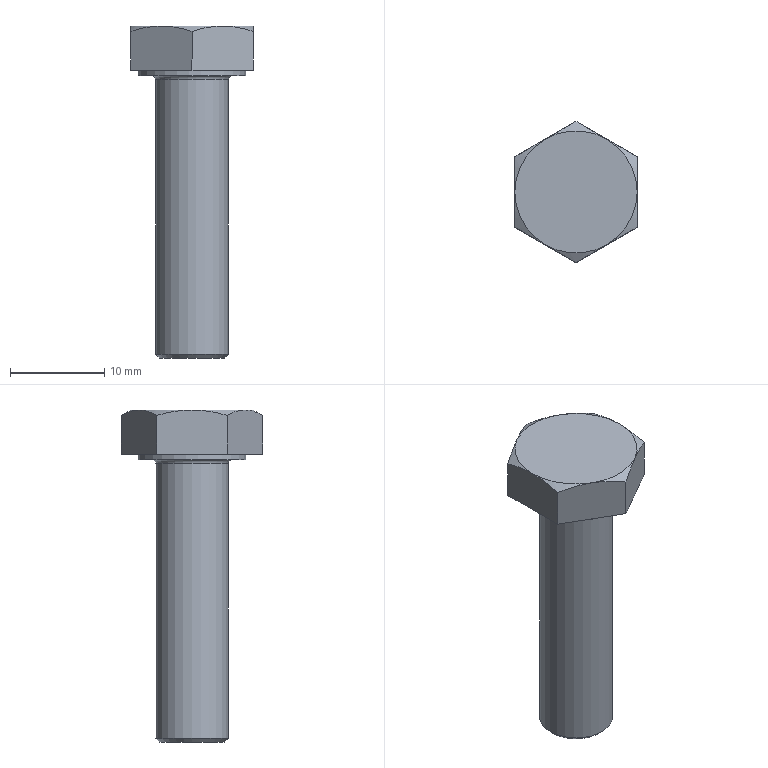Part | NX | features SKETCH 4, EXTRUDE 3, META 3, DATUM_CSYS 2, BLEND 1, CHAMFER 1, LINE 1, SWP104 1, SYMBOLIC_THREAD 1, THREADS 1 | 1 solid | 20 faces | box 13 x 15.011 x 35.3 mm | volume 2165 mm3 | plane 10 | cone 7 | cylinder 2 | torus 1 | commonest cylinder face diameters 7.76 x1 11.47 x1
STEP:
#1=CARTESIAN_POINT('',(4.28,0.,0.));
#2=VERTEX_POINT('',#1);
#3=CARTESIAN_POINT('',(0.,0.,0.));
#4=DIRECTION('',(0.,0.,1.));
#5=DIRECTION('',(1.,0.,0.));
#6=AXIS2_PLACEMENT_3D('',#3,#4,#5);
#7=CIRCLE('',#6,4.28);
#8=EDGE_CURVE('',#2,#2,#7,.T.);
#9=ORIENTED_EDGE('',*,*,#8,.T.);
#10=EDGE_LOOP('',(#9));
#11=FACE_BOUND('',#10,.T.);
#12=CARTESIAN_POINT('',(5.735,0.,0.));
#13=VERTEX_POINT('',#12);
#14=CARTESIAN_POINT('',(0.,0.,0.));
#15=DIRECTION('',(0.,0.,1.));
#16=DIRECTION('',(1.,0.,0.));
#17=AXIS2_PLACEMENT_3D('',#14,#15,#16);
#18=CIRCLE('',#17,5.735);
#19=EDGE_CURVE('',#13,#13,#18,.T.);
#20=ORIENTED_EDGE('',*,*,#19,.F.);
#21=EDGE_LOOP('',(#20));
#22=FACE_BOUND('',#21,.T.);
#23=CARTESIAN_POINT('',(0.,0.,0.));
#24=DIRECTION('',(0.,0.,1.));
#25=DIRECTION('',(1.,0.,0.));
#26=AXIS2_PLACEMENT_3D('',#23,#24,#25);
#27=PLANE('',#26);
#28=ADVANCED_FACE('',(#11,#22),#27,.F.);
#29=CARTESIAN_POINT('',(6.5,3.753,4.719));
#30=VERTEX_POINT('',#29);
#31=CARTESIAN_POINT('',(3.25,5.629,5.3));
#32=VERTEX_POINT('',#31);
#33=CARTESIAN_POINT('',(6.5,3.753,4.719));
#34=CARTESIAN_POINT('',(5.437,4.367,5.074));
#35=CARTESIAN_POINT('',(4.357,4.99,5.3));
#36=CARTESIAN_POINT('',(3.25,5.629,5.3));
#37=B_SPLINE_CURVE_WITH_KNOTS('',3,(#33,#34,#35,#36),.UNSPECIFIED.,.F.,.F.,(4,4),(0.000000238,0.003797),.UNSPECIFIED.);
#38=EDGE_CURVE('',#30,#32,#37,.T.);
#39=ORIENTED_EDGE('',*,*,#38,.F.);
#40=CARTESIAN_POINT('',(6.5,3.753,0.6));
#41=VERTEX_POINT('',#40);
#42=CARTESIAN_POINT('',(6.5,3.753,5.3));
#43=DIRECTION('',(0.,0.,-1.));
#44=VECTOR('',#43,1000.);
#45=LINE('',#42,#44);
#46=EDGE_CURVE('',#30,#41,#45,.T.);
#47=ORIENTED_EDGE('',*,*,#46,.T.);
#48=CARTESIAN_POINT('',(0.,7.506,0.6));
#49=VERTEX_POINT('',#48);
#50=CARTESIAN_POINT('',(0.,7.506,0.6));
#51=DIRECTION('',(0.866,-0.5,0.));
#52=VECTOR('',#51,1000.);
#53=LINE('',#50,#52);
#54=EDGE_CURVE('',#49,#41,#53,.T.);
#55=ORIENTED_EDGE('',*,*,#54,.F.);
#56=CARTESIAN_POINT('',(0.,7.506,4.719));
#57=VERTEX_POINT('',#56);
#58=CARTESIAN_POINT('',(0.,7.506,5.3));
#59=DIRECTION('',(0.,0.,-1.));
#60=VECTOR('',#59,1000.);
#61=LINE('',#58,#60);
#62=EDGE_CURVE('',#57,#49,#61,.T.);
#63=ORIENTED_EDGE('',*,*,#62,.F.);
#64=CARTESIAN_POINT('',(3.25,5.629,5.3));
#65=CARTESIAN_POINT('',(2.147,6.266,5.3));
#66=CARTESIAN_POINT('',(1.061,6.893,5.073));
#67=CARTESIAN_POINT('',(0.,7.506,4.719));
#68=B_SPLINE_CURVE_WITH_KNOTS('',3,(#64,#65,#66,#67),.UNSPECIFIED.,.F.,.F.,(4,4),(0.003797,0.00758),.UNSPECIFIED.);
#69=EDGE_CURVE('',#32,#57,#68,.T.);
#70=ORIENTED_EDGE('',*,*,#69,.F.);
#71=EDGE_LOOP('',(#39,#47,#55,#63,#70));
#72=FACE_BOUND('',#71,.T.);
#73=CARTESIAN_POINT('',(0.,7.506,5.3));
#74=DIRECTION('',(0.5,0.866,0.));
#75=DIRECTION('',(-0.866,0.5,0.));
#76=AXIS2_PLACEMENT_3D('',#73,#74,#75);
#77=PLANE('',#76);
#78=ADVANCED_FACE('',(#72),#77,.T.);
#79=CARTESIAN_POINT('',(6.5,-3.753,4.719));
#80=VERTEX_POINT('',#79);
#81=CARTESIAN_POINT('',(6.5,0.,5.3));
#82=VERTEX_POINT('',#81);
#83=CARTESIAN_POINT('',(6.5,-3.753,4.719));
#84=CARTESIAN_POINT('',(6.5,-2.532,5.072));
#85=CARTESIAN_POINT('',(6.5,-1.268,5.3));
#86=CARTESIAN_POINT('',(6.5,0.,5.3));
#87=B_SPLINE_CURVE_WITH_KNOTS('',3,(#83,#84,#85,#86),.UNSPECIFIED.,.F.,.F.,(4,4),(0.006695,0.01049),.UNSPECIFIED.);
#88=EDGE_CURVE('',#80,#82,#87,.T.);
#89=ORIENTED_EDGE('',*,*,#88,.F.);
#90=CARTESIAN_POINT('',(6.5,-3.753,0.6));
#91=VERTEX_POINT('',#90);
#92=CARTESIAN_POINT('',(6.5,-3.753,5.3));
#93=DIRECTION('',(0.,0.,-1.));
#94=VECTOR('',#93,1000.);
#95=LINE('',#92,#94);
#96=EDGE_CURVE('',#80,#91,#95,.T.);
#97=ORIENTED_EDGE('',*,*,#96,.T.);
#98=CARTESIAN_POINT('',(6.5,3.753,0.6));
#99=DIRECTION('',(0.,-1.,0.));
#100=VECTOR('',#99,1000.);
#101=LINE('',#98,#100);
#102=EDGE_CURVE('',#41,#91,#101,.T.);
#103=ORIENTED_EDGE('',*,*,#102,.F.);
#104=ORIENTED_EDGE('',*,*,#46,.F.);
#105=CARTESIAN_POINT('',(6.5,0.,5.3));
#106=CARTESIAN_POINT('',(6.5,1.269,5.3));
#107=CARTESIAN_POINT('',(6.5,2.539,5.07));
#108=CARTESIAN_POINT('',(6.5,3.753,4.719));
#109=B_SPLINE_CURVE_WITH_KNOTS('',3,(#105,#106,#107,#108),.UNSPECIFIED.,.F.,.F.,(4,4),(0.01049,0.01429),.UNSPECIFIED.);
#110=EDGE_CURVE('',#82,#30,#109,.T.);
#111=ORIENTED_EDGE('',*,*,#110,.F.);
#112=EDGE_LOOP('',(#89,#97,#103,#104,#111));
#113=FACE_BOUND('',#112,.T.);
#114=CARTESIAN_POINT('',(6.5,3.753,5.3));
#115=DIRECTION('',(1.,0.,0.));
#116=DIRECTION('',(0.,0.,-1.));
#117=AXIS2_PLACEMENT_3D('',#114,#115,#116);
#118=PLANE('',#117);
#119=ADVANCED_FACE('',(#113),#118,.T.);
#120=CARTESIAN_POINT('',(0.,-7.506,4.719));
#121=VERTEX_POINT('',#120);
#122=CARTESIAN_POINT('',(3.25,-5.629,5.3));
#123=VERTEX_POINT('',#122);
#124=CARTESIAN_POINT('',(0.,-7.506,4.719));
#125=CARTESIAN_POINT('',(1.063,-6.892,5.074));
#126=CARTESIAN_POINT('',(2.143,-6.269,5.3));
#127=CARTESIAN_POINT('',(3.25,-5.629,5.3));
#128=B_SPLINE_CURVE_WITH_KNOTS('',3,(#124,#125,#126,#127),.UNSPECIFIED.,.F.,.F.,(4,4),(0.000000238,0.003797),.UNSPECIFIED.);
#129=EDGE_CURVE('',#121,#123,#128,.T.);
#130=ORIENTED_EDGE('',*,*,#129,.F.);
#131=CARTESIAN_POINT('',(0.,-7.506,0.6));
#132=VERTEX_POINT('',#131);
#133=CARTESIAN_POINT('',(0.,-7.506,5.3));
#134=DIRECTION('',(0.,0.,-1.));
#135=VECTOR('',#134,1000.);
#136=LINE('',#133,#135);
#137=EDGE_CURVE('',#121,#132,#136,.T.);
#138=ORIENTED_EDGE('',*,*,#137,.T.);
#139=CARTESIAN_POINT('',(6.5,-3.753,0.6));
#140=DIRECTION('',(-0.866,-0.5,0.));
#141=VECTOR('',#140,1000.);
#142=LINE('',#139,#141);
#143=EDGE_CURVE('',#91,#132,#142,.T.);
#144=ORIENTED_EDGE('',*,*,#143,.F.);
#145=ORIENTED_EDGE('',*,*,#96,.F.);
#146=CARTESIAN_POINT('',(3.25,-5.629,5.3));
#147=CARTESIAN_POINT('',(4.353,-4.992,5.3));
#148=CARTESIAN_POINT('',(5.439,-4.365,5.073));
#149=CARTESIAN_POINT('',(6.5,-3.753,4.719));
#150=B_SPLINE_CURVE_WITH_KNOTS('',3,(#146,#147,#148,#149),.UNSPECIFIED.,.F.,.F.,(4,4),(0.003797,0.00758),.UNSPECIFIED.);
#151=EDGE_CURVE('',#123,#80,#150,.T.);
#152=ORIENTED_EDGE('',*,*,#151,.F.);
#153=EDGE_LOOP('',(#130,#138,#144,#145,#152));
#154=FACE_BOUND('',#153,.T.);
#155=CARTESIAN_POINT('',(6.5,-3.753,5.3));
#156=DIRECTION('',(0.5,-0.866,0.));
#157=DIRECTION('',(0.866,0.5,0.));
#158=AXIS2_PLACEMENT_3D('',#155,#156,#157);
#159=PLANE('',#158);
#160=ADVANCED_FACE('',(#154),#159,.T.);
#161=CARTESIAN_POINT('',(-6.5,-3.753,4.719));
#162=VERTEX_POINT('',#161);
#163=CARTESIAN_POINT('',(-3.25,-5.629,5.3));
#164=VERTEX_POINT('',#163);
#165=CARTESIAN_POINT('',(-6.5,-3.753,4.719));
#166=CARTESIAN_POINT('',(-5.437,-4.367,5.074));
#167=CARTESIAN_POINT('',(-4.357,-4.99,5.3));
#168=CARTESIAN_POINT('',(-3.25,-5.629,5.3));
#169=B_SPLINE_CURVE_WITH_KNOTS('',3,(#165,#166,#167,#168),.UNSPECIFIED.,.F.,.F.,(4,4),(0.000000238,0.003797),.UNSPECIFIED.);
#170=EDGE_CURVE('',#162,#164,#169,.T.);
#171=ORIENTED_EDGE('',*,*,#170,.F.);
#172=CARTESIAN_POINT('',(-6.5,-3.753,0.6));
#173=VERTEX_POINT('',#172);
#174=CARTESIAN_POINT('',(-6.5,-3.753,5.3));
#175=DIRECTION('',(0.,0.,-1.));
#176=VECTOR('',#175,1000.);
#177=LINE('',#174,#176);
#178=EDGE_CURVE('',#162,#173,#177,.T.);
#179=ORIENTED_EDGE('',*,*,#178,.T.);
#180=CARTESIAN_POINT('',(0.,-7.506,0.6));
#181=DIRECTION('',(-0.866,0.5,0.));
#182=VECTOR('',#181,1000.);
#183=LINE('',#180,#182);
#184=EDGE_CURVE('',#132,#173,#183,.T.);
#185=ORIENTED_EDGE('',*,*,#184,.F.);
#186=ORIENTED_EDGE('',*,*,#137,.F.);
#187=CARTESIAN_POINT('',(-3.25,-5.629,5.3));
#188=CARTESIAN_POINT('',(-2.147,-6.266,5.3));
#189=CARTESIAN_POINT('',(-1.061,-6.893,5.073));
#190=CARTESIAN_POINT('',(0.,-7.506,4.719));
#191=B_SPLINE_CURVE_WITH_KNOTS('',3,(#187,#188,#189,#190),.UNSPECIFIED.,.F.,.F.,(4,4),(0.003797,0.00758),.UNSPECIFIED.);
#192=EDGE_CURVE('',#164,#121,#191,.T.);
#193=ORIENTED_EDGE('',*,*,#192,.F.);
#194=EDGE_LOOP('',(#171,#179,#185,#186,#193));
#195=FACE_BOUND('',#194,.T.);
#196=CARTESIAN_POINT('',(0.,-7.506,5.3));
#197=DIRECTION('',(-0.5,-0.866,0.));
#198=DIRECTION('',(0.866,-0.5,0.));
#199=AXIS2_PLACEMENT_3D('',#196,#197,#198);
#200=PLANE('',#199);
#201=ADVANCED_FACE('',(#195),#200,.T.);
#202=CARTESIAN_POINT('',(-6.5,3.753,4.719));
#203=VERTEX_POINT('',#202);
#204=CARTESIAN_POINT('',(-6.5,0.,5.3));
#205=VERTEX_POINT('',#204);
#206=CARTESIAN_POINT('',(-6.5,0.,5.3));
#207=CARTESIAN_POINT('',(-6.5,1.269,5.3));
#208=CARTESIAN_POINT('',(-6.5,2.539,5.07));
#209=CARTESIAN_POINT('',(-6.5,3.753,4.719));
#210=B_SPLINE_CURVE_WITH_KNOTS('',3,(#206,#207,#208,#209),.UNSPECIFIED.,.F.,.F.,(4,4),(0.01049,0.01429),.UNSPECIFIED.);
#211=EDGE_CURVE('',#203,#205,#210,.F.);
#212=ORIENTED_EDGE('',*,*,#211,.F.);
#213=CARTESIAN_POINT('',(-6.5,3.753,0.6));
#214=VERTEX_POINT('',#213);
#215=CARTESIAN_POINT('',(-6.5,3.753,5.3));
#216=DIRECTION('',(0.,0.,-1.));
#217=VECTOR('',#216,1000.);
#218=LINE('',#215,#217);
#219=EDGE_CURVE('',#203,#214,#218,.T.);
#220=ORIENTED_EDGE('',*,*,#219,.T.);
#221=CARTESIAN_POINT('',(-6.5,-3.753,0.6));
#222=DIRECTION('',(0.,1.,0.));
#223=VECTOR('',#222,1000.);
#224=LINE('',#221,#223);
#225=EDGE_CURVE('',#173,#214,#224,.T.);
#226=ORIENTED_EDGE('',*,*,#225,.F.);
#227=ORIENTED_EDGE('',*,*,#178,.F.);
#228=CARTESIAN_POINT('',(-6.5,-3.753,4.719));
#229=CARTESIAN_POINT('',(-6.5,-2.532,5.072));
#230=CARTESIAN_POINT('',(-6.5,-1.268,5.3));
#231=CARTESIAN_POINT('',(-6.5,0.,5.3));
#232=B_SPLINE_CURVE_WITH_KNOTS('',3,(#228,#229,#230,#231),.UNSPECIFIED.,.F.,.F.,(4,4),(0.006695,0.01049),.UNSPECIFIED.);
#233=EDGE_CURVE('',#205,#162,#232,.F.);
#234=ORIENTED_EDGE('',*,*,#233,.F.);
#235=EDGE_LOOP('',(#212,#220,#226,#227,#234));
#236=FACE_BOUND('',#235,.T.);
#237=CARTESIAN_POINT('',(-6.5,-3.753,5.3));
#238=DIRECTION('',(-1.,0.,0.));
#239=DIRECTION('',(0.,0.,1.));
#240=AXIS2_PLACEMENT_3D('',#237,#238,#239);
#241=PLANE('',#240);
#242=ADVANCED_FACE('',(#236),#241,.T.);
#243=CARTESIAN_POINT('',(-3.25,5.629,5.3));
#244=VERTEX_POINT('',#243);
#245=CARTESIAN_POINT('',(0.,7.506,4.719));
#246=CARTESIAN_POINT('',(-1.063,6.892,5.074));
#247=CARTESIAN_POINT('',(-2.143,6.269,5.3));
#248=CARTESIAN_POINT('',(-3.25,5.629,5.3));
#249=B_SPLINE_CURVE_WITH_KNOTS('',3,(#245,#246,#247,#248),.UNSPECIFIED.,.F.,.F.,(4,4),(0.000000238,0.003797),.UNSPECIFIED.);
#250=EDGE_CURVE('',#57,#244,#249,.T.);
#251=ORIENTED_EDGE('',*,*,#250,.F.);
#252=ORIENTED_EDGE('',*,*,#62,.T.);
#253=CARTESIAN_POINT('',(-6.5,3.753,0.6));
#254=DIRECTION('',(0.866,0.5,0.));
#255=VECTOR('',#254,1000.);
#256=LINE('',#253,#255);
#257=EDGE_CURVE('',#214,#49,#256,.T.);
#258=ORIENTED_EDGE('',*,*,#257,.F.);
#259=ORIENTED_EDGE('',*,*,#219,.F.);
#260=CARTESIAN_POINT('',(-3.25,5.629,5.3));
#261=CARTESIAN_POINT('',(-4.353,4.992,5.3));
#262=CARTESIAN_POINT('',(-5.439,4.365,5.073));
#263=CARTESIAN_POINT('',(-6.5,3.753,4.719));
#264=B_SPLINE_CURVE_WITH_KNOTS('',3,(#260,#261,#262,#263),.UNSPECIFIED.,.F.,.F.,(4,4),(0.003797,0.00758),.UNSPECIFIED.);
#265=EDGE_CURVE('',#244,#203,#264,.T.);
#266=ORIENTED_EDGE('',*,*,#265,.F.);
#267=EDGE_LOOP('',(#251,#252,#258,#259,#266));
#268=FACE_BOUND('',#267,.T.);
#269=CARTESIAN_POINT('',(-6.5,3.753,5.3));
#270=DIRECTION('',(-0.5,0.866,0.));
#271=DIRECTION('',(-0.866,-0.5,0.));
#272=AXIS2_PLACEMENT_3D('',#269,#270,#271);
#273=PLANE('',#272);
#274=ADVANCED_FACE('',(#268),#273,.T.);
#275=CARTESIAN_POINT('',(5.735,0.,0.6));
#276=VERTEX_POINT('',#275);
#277=CARTESIAN_POINT('',(0.,0.,0.6));
#278=DIRECTION('',(0.,0.,1.));
#279=DIRECTION('',(1.,0.,0.));
#280=AXIS2_PLACEMENT_3D('',#277,#278,#279);
#281=CIRCLE('',#280,5.735);
#282=EDGE_CURVE('',#276,#276,#281,.T.);
#283=ORIENTED_EDGE('',*,*,#282,.T.);
#284=EDGE_LOOP('',(#283));
#285=FACE_BOUND('',#284,.T.);
#286=ORIENTED_EDGE('',*,*,#54,.T.);
#287=ORIENTED_EDGE('',*,*,#102,.T.);
#288=ORIENTED_EDGE('',*,*,#143,.T.);
#289=ORIENTED_EDGE('',*,*,#184,.T.);
#290=ORIENTED_EDGE('',*,*,#225,.T.);
#291=ORIENTED_EDGE('',*,*,#257,.T.);
#292=EDGE_LOOP('',(#286,#287,#288,#289,#290,#291));
#293=FACE_BOUND('',#292,.T.);
#294=CARTESIAN_POINT('',(0.,7.506,0.6));
#295=DIRECTION('',(0.,0.,1.));
#296=DIRECTION('',(1.,0.,0.));
#297=AXIS2_PLACEMENT_3D('',#294,#295,#296);
#298=PLANE('',#297);
#299=ADVANCED_FACE('',(#285,#293),#298,.F.);
#300=ORIENTED_EDGE('',*,*,#282,.F.);
#301=EDGE_LOOP('',(#300));
#302=FACE_BOUND('',#301,.T.);
#303=ORIENTED_EDGE('',*,*,#19,.T.);
#304=EDGE_LOOP('',(#303));
#305=FACE_BOUND('',#304,.T.);
#306=CARTESIAN_POINT('',(0.,0.,0.6));
#307=DIRECTION('',(0.,0.,-1.));
#308=DIRECTION('',(-1.,0.,0.));
#309=AXIS2_PLACEMENT_3D('',#306,#307,#308);
#310=CYLINDRICAL_SURFACE('',#309,5.735);
#311=ADVANCED_FACE('',(#302,#305),#310,.T.);
#312=CARTESIAN_POINT('',(-3.88,0.,-29.612));
#313=VERTEX_POINT('',#312);
#314=CARTESIAN_POINT('',(0.,0.,-29.612));
#315=DIRECTION('',(0.,0.,-1.));
#316=DIRECTION('',(-1.,0.,0.));
#317=AXIS2_PLACEMENT_3D('',#314,#315,#316);
#318=CIRCLE('',#317,3.88);
#319=EDGE_CURVE('',#313,#313,#318,.F.);
#320=ORIENTED_EDGE('',*,*,#319,.T.);
#321=EDGE_LOOP('',(#320));
#322=FACE_BOUND('',#321,.T.);
#323=CARTESIAN_POINT('',(3.88,0.,-0.4));
#324=VERTEX_POINT('',#323);
#325=CARTESIAN_POINT('',(0.,0.,-0.4));
#326=DIRECTION('',(0.,0.,1.));
#327=DIRECTION('',(1.,0.,0.));
#328=AXIS2_PLACEMENT_3D('',#325,#326,#327);
#329=CIRCLE('',#328,3.88);
#330=EDGE_CURVE('',#324,#324,#329,.F.);
#331=ORIENTED_EDGE('',*,*,#330,.T.);
#332=EDGE_LOOP('',(#331));
#333=FACE_BOUND('',#332,.T.);
#334=CARTESIAN_POINT('',(0.,0.,-30.));
#335=DIRECTION('',(0.,0.,1.));
#336=DIRECTION('',(1.,0.,0.));
#337=AXIS2_PLACEMENT_3D('',#334,#335,#336);
#338=CYLINDRICAL_SURFACE('',#337,3.88);
#339=ADVANCED_FACE('',(#322,#333),#338,.T.);
#340=CARTESIAN_POINT('',(-3.492,0.,-30.));
#341=VERTEX_POINT('',#340);
#342=CARTESIAN_POINT('',(0.,0.,-30.));
#343=DIRECTION('',(0.,0.,-1.));
#344=DIRECTION('',(-1.,0.,0.));
#345=AXIS2_PLACEMENT_3D('',#342,#343,#344);
#346=CIRCLE('',#345,3.492);
#347=EDGE_CURVE('',#341,#341,#346,.T.);
#348=ORIENTED_EDGE('',*,*,#347,.T.);
#349=EDGE_LOOP('',(#348));
#350=FACE_BOUND('',#349,.T.);
#351=CARTESIAN_POINT('',(0.,0.,-30.));
#352=DIRECTION('',(0.,0.,-1.));
#353=DIRECTION('',(-1.,0.,0.));
#354=AXIS2_PLACEMENT_3D('',#351,#352,#353);
#355=PLANE('',#354);
#356=ADVANCED_FACE('',(#350),#355,.T.);
#357=ORIENTED_EDGE('',*,*,#211,.T.);
#358=CARTESIAN_POINT('',(0.,0.,5.3));
#359=DIRECTION('',(0.,0.,-1.));
#360=DIRECTION('',(-1.,0.,0.));
#361=AXIS2_PLACEMENT_3D('',#358,#359,#360);
#362=CIRCLE('',#361,6.5);
#363=EDGE_CURVE('',#205,#244,#362,.T.);
#364=ORIENTED_EDGE('',*,*,#363,.T.);
#365=ORIENTED_EDGE('',*,*,#265,.T.);
#366=EDGE_LOOP('',(#357,#364,#365));
#367=FACE_BOUND('',#366,.T.);
#368=CARTESIAN_POINT('',(0.,0.,5.3));
#369=DIRECTION('',(0.,0.,-1.));
#370=DIRECTION('',(-1.,0.,0.));
#371=AXIS2_PLACEMENT_3D('',#368,#369,#370);
#372=CONICAL_SURFACE('',#371,6.5,1.047);
#373=ADVANCED_FACE('',(#367),#372,.T.);
#374=ORIENTED_EDGE('',*,*,#69,.T.);
#375=ORIENTED_EDGE('',*,*,#250,.T.);
#376=CARTESIAN_POINT('',(0.,0.,5.3));
#377=DIRECTION('',(0.,0.,-1.));
#378=DIRECTION('',(-1.,0.,0.));
#379=AXIS2_PLACEMENT_3D('',#376,#377,#378);
#380=CIRCLE('',#379,6.5);
#381=EDGE_CURVE('',#244,#32,#380,.T.);
#382=ORIENTED_EDGE('',*,*,#381,.T.);
#383=EDGE_LOOP('',(#374,#375,#382));
#384=FACE_BOUND('',#383,.T.);
#385=CARTESIAN_POINT('',(0.,0.,5.3));
#386=DIRECTION('',(0.,0.,-1.));
#387=DIRECTION('',(-1.,0.,0.));
#388=AXIS2_PLACEMENT_3D('',#385,#386,#387);
#389=CONICAL_SURFACE('',#388,6.5,1.047);
#390=ADVANCED_FACE('',(#384),#389,.T.);
#391=ORIENTED_EDGE('',*,*,#170,.T.);
#392=CARTESIAN_POINT('',(0.,0.,5.3));
#393=DIRECTION('',(0.,0.,-1.));
#394=DIRECTION('',(-1.,0.,0.));
#395=AXIS2_PLACEMENT_3D('',#392,#393,#394);
#396=CIRCLE('',#395,6.5);
#397=EDGE_CURVE('',#164,#205,#396,.T.);
#398=ORIENTED_EDGE('',*,*,#397,.T.);
#399=ORIENTED_EDGE('',*,*,#233,.T.);
#400=EDGE_LOOP('',(#391,#398,#399));
#401=FACE_BOUND('',#400,.T.);
#402=CARTESIAN_POINT('',(0.,0.,5.3));
#403=DIRECTION('',(0.,0.,-1.));
#404=DIRECTION('',(-1.,0.,0.));
#405=AXIS2_PLACEMENT_3D('',#402,#403,#404);
#406=CONICAL_SURFACE('',#405,6.5,1.047);
#407=ADVANCED_FACE('',(#401),#406,.T.);
#408=ORIENTED_EDGE('',*,*,#129,.T.);
#409=CARTESIAN_POINT('',(0.,0.,5.3));
#410=DIRECTION('',(0.,0.,-1.));
#411=DIRECTION('',(-1.,0.,0.));
#412=AXIS2_PLACEMENT_3D('',#409,#410,#411);
#413=CIRCLE('',#412,6.5);
#414=EDGE_CURVE('',#123,#164,#413,.T.);
#415=ORIENTED_EDGE('',*,*,#414,.T.);
#416=ORIENTED_EDGE('',*,*,#192,.T.);
#417=EDGE_LOOP('',(#408,#415,#416));
#418=FACE_BOUND('',#417,.T.);
#419=CARTESIAN_POINT('',(0.,0.,5.3));
#420=DIRECTION('',(0.,0.,-1.));
#421=DIRECTION('',(-1.,0.,0.));
#422=AXIS2_PLACEMENT_3D('',#419,#420,#421);
#423=CONICAL_SURFACE('',#422,6.5,1.047);
#424=ADVANCED_FACE('',(#418),#423,.T.);
#425=ORIENTED_EDGE('',*,*,#151,.T.);
#426=ORIENTED_EDGE('',*,*,#88,.T.);
#427=CARTESIAN_POINT('',(0.,0.,5.3));
#428=DIRECTION('',(0.,0.,-1.));
#429=DIRECTION('',(-1.,0.,0.));
#430=AXIS2_PLACEMENT_3D('',#427,#428,#429);
#431=CIRCLE('',#430,6.5);
#432=EDGE_CURVE('',#82,#123,#431,.T.);
#433=ORIENTED_EDGE('',*,*,#432,.T.);
#434=EDGE_LOOP('',(#425,#426,#433));
#435=FACE_BOUND('',#434,.T.);
#436=CARTESIAN_POINT('',(0.,0.,5.3));
#437=DIRECTION('',(0.,0.,-1.));
#438=DIRECTION('',(-1.,0.,0.));
#439=AXIS2_PLACEMENT_3D('',#436,#437,#438);
#440=CONICAL_SURFACE('',#439,6.5,1.047);
#441=ADVANCED_FACE('',(#435),#440,.T.);
#442=ORIENTED_EDGE('',*,*,#110,.T.);
#443=ORIENTED_EDGE('',*,*,#38,.T.);
#444=CARTESIAN_POINT('',(0.,0.,5.3));
#445=DIRECTION('',(0.,0.,-1.));
#446=DIRECTION('',(-1.,0.,0.));
#447=AXIS2_PLACEMENT_3D('',#444,#445,#446);
#448=CIRCLE('',#447,6.5);
#449=EDGE_CURVE('',#32,#82,#448,.T.);
#450=ORIENTED_EDGE('',*,*,#449,.T.);
#451=EDGE_LOOP('',(#442,#443,#450));
#452=FACE_BOUND('',#451,.T.);
#453=CARTESIAN_POINT('',(0.,0.,5.3));
#454=DIRECTION('',(0.,0.,-1.));
#455=DIRECTION('',(-1.,0.,0.));
#456=AXIS2_PLACEMENT_3D('',#453,#454,#455);
#457=CONICAL_SURFACE('',#456,6.5,1.047);
#458=ADVANCED_FACE('',(#452),#457,.T.);
#459=ORIENTED_EDGE('',*,*,#363,.F.);
#460=ORIENTED_EDGE('',*,*,#397,.F.);
#461=ORIENTED_EDGE('',*,*,#414,.F.);
#462=ORIENTED_EDGE('',*,*,#432,.F.);
#463=ORIENTED_EDGE('',*,*,#449,.F.);
#464=ORIENTED_EDGE('',*,*,#381,.F.);
#465=EDGE_LOOP('',(#459,#460,#461,#462,#463,#464));
#466=FACE_BOUND('',#465,.T.);
#467=CARTESIAN_POINT('',(0.,7.506,5.3));
#468=DIRECTION('',(0.,0.,1.));
#469=DIRECTION('',(1.,0.,0.));
#470=AXIS2_PLACEMENT_3D('',#467,#468,#469);
#471=PLANE('',#470);
#472=ADVANCED_FACE('',(#466),#471,.T.);
#473=ORIENTED_EDGE('',*,*,#8,.F.);
#474=EDGE_LOOP('',(#473));
#475=FACE_BOUND('',#474,.T.);
#476=ORIENTED_EDGE('',*,*,#330,.F.);
#477=EDGE_LOOP('',(#476));
#478=FACE_BOUND('',#477,.T.);
#479=CARTESIAN_POINT('',(0.,0.,-0.4));
#480=DIRECTION('',(0.,0.,1.));
#481=DIRECTION('',(1.,0.,0.));
#482=AXIS2_PLACEMENT_3D('',#479,#480,#481);
#483=TOROIDAL_SURFACE('',#482,4.28,0.4);
#484=ADVANCED_FACE('',(#475,#478),#483,.F.);
#485=ORIENTED_EDGE('',*,*,#319,.F.);
#486=EDGE_LOOP('',(#485));
#487=FACE_BOUND('',#486,.T.);
#488=ORIENTED_EDGE('',*,*,#347,.F.);
#489=EDGE_LOOP('',(#488));
#490=FACE_BOUND('',#489,.T.);
#491=CARTESIAN_POINT('',(0.,0.,-30.));
#492=DIRECTION('',(0.,0.,1.));
#493=DIRECTION('',(1.,0.,0.));
#494=AXIS2_PLACEMENT_3D('',#491,#492,#493);
#495=CONICAL_SURFACE('',#494,3.492,0.7854);
#496=ADVANCED_FACE('',(#487,#490),#495,.T.);
#497=CLOSED_SHELL('',(#28,#78,#119,#160,#201,#242,#274,#299,#311,#339,#356,#373,#390,#407,#424,#441,#458,#472,#484,#496));
#498=MANIFOLD_SOLID_BREP('',#497);
#499=(LENGTH_UNIT()NAMED_UNIT(*)SI_UNIT(.MILLI.,.METRE.));
#500=UNCERTAINTY_MEASURE_WITH_UNIT(LENGTH_MEASURE(0.0508),#499,'','');
#501=(NAMED_UNIT(*)PLANE_ANGLE_UNIT()SI_UNIT($,.RADIAN.));
#502=(NAMED_UNIT(*)SI_UNIT($,.STERADIAN.)SOLID_ANGLE_UNIT());
#503=(GEOMETRIC_REPRESENTATION_CONTEXT(3)GLOBAL_UNCERTAINTY_ASSIGNED_CONTEXT((#500))GLOBAL_UNIT_ASSIGNED_CONTEXT((#499,#501,#502))REPRESENTATION_CONTEXT('',''));
#504=ADVANCED_BREP_SHAPE_REPRESENTATION('',(#498),#503);